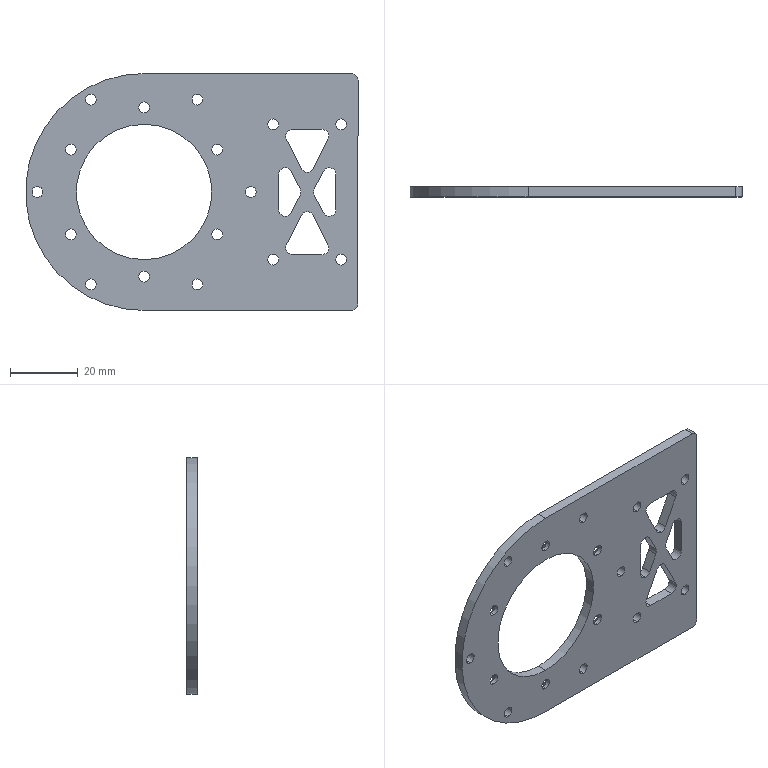Part | SolidWorks | features ICE 2, 3DProfileFeature 1, Extrusion 1, Fillet 1, HoleWzd 1 | 1 solid | 81 faces | box 98.2 x 3 x 70 mm | volume 13699 mm3 | cylinder 52 | plane 17 | cone 12 | commonest cylinder face diameters 3.2 x32 4 x17 40 x2 70 x1